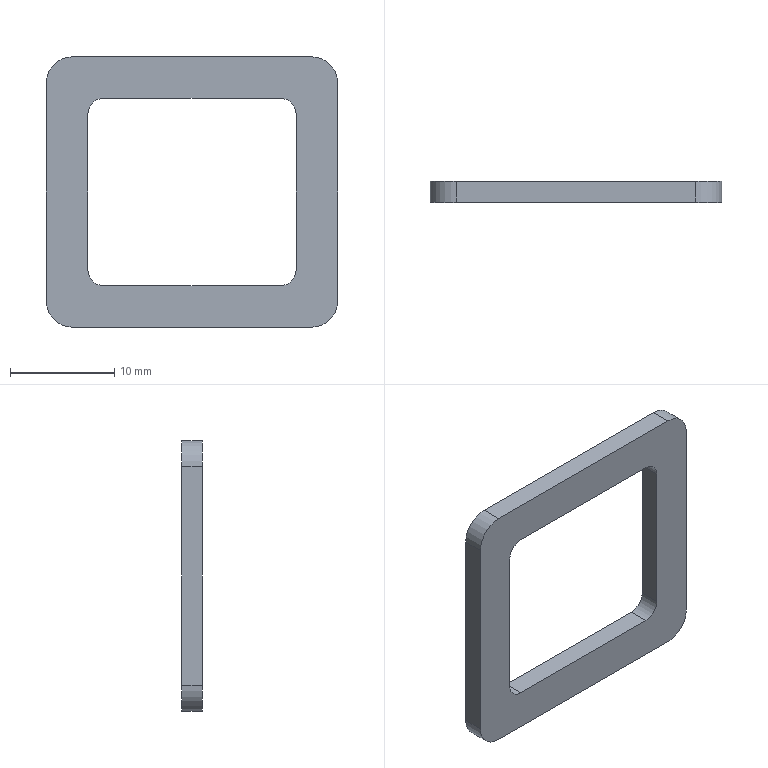Part | STEP file | 10000020460swp000-1 | 1 solid | 18 faces | box 28 x 2 x 26 mm | volume 729.133 mm3 | plane 10 | cylinder 8 | commonest cylinder face diameters 3 x4 5 x4
STEP:
#1=CARTESIAN_POINT('',(14.,2.,10.5));
#2=VERTEX_POINT('',#1);
#3=CARTESIAN_POINT('',(14.,2.,-10.5));
#4=VERTEX_POINT('',#3);
#5=CARTESIAN_POINT('',(14.,2.,-13.));
#6=DIRECTION('',(0.,0.,-1.));
#7=VECTOR('',#6,1000.);
#8=LINE('',#5,#7);
#9=EDGE_CURVE('',#2,#4,#8,.T.);
#10=ORIENTED_EDGE('',*,*,#9,.F.);
#11=CARTESIAN_POINT('',(14.,0.,10.5));
#12=VERTEX_POINT('',#11);
#13=CARTESIAN_POINT('',(14.,2.,10.5));
#14=DIRECTION('',(0.,-1.,0.));
#15=VECTOR('',#14,1000.);
#16=LINE('',#13,#15);
#17=EDGE_CURVE('',#2,#12,#16,.T.);
#18=ORIENTED_EDGE('',*,*,#17,.T.);
#19=CARTESIAN_POINT('',(14.,0.,-10.5));
#20=VERTEX_POINT('',#19);
#21=CARTESIAN_POINT('',(14.,0.,-13.));
#22=DIRECTION('',(0.,0.,-1.));
#23=VECTOR('',#22,1000.);
#24=LINE('',#21,#23);
#25=EDGE_CURVE('',#12,#20,#24,.T.);
#26=ORIENTED_EDGE('',*,*,#25,.T.);
#27=CARTESIAN_POINT('',(14.,2.,-10.5));
#28=DIRECTION('',(0.,1.,0.));
#29=VECTOR('',#28,1000.);
#30=LINE('',#27,#29);
#31=EDGE_CURVE('',#20,#4,#30,.T.);
#32=ORIENTED_EDGE('',*,*,#31,.T.);
#33=EDGE_LOOP('',(#10,#18,#26,#32));
#34=FACE_OUTER_BOUND('',#33,.T.);
#35=CARTESIAN_POINT('',(14.,2.,-13.));
#36=DIRECTION('',(-1.,0.,0.));
#37=DIRECTION('',(0.,0.,1.));
#38=AXIS2_PLACEMENT_3D('',#35,#36,#37);
#39=PLANE('',#38);
#40=ADVANCED_FACE('',(#34),#39,.F.);
#41=CARTESIAN_POINT('',(11.5,2.,-13.));
#42=VERTEX_POINT('',#41);
#43=CARTESIAN_POINT('',(-11.5,2.,-13.));
#44=VERTEX_POINT('',#43);
#45=CARTESIAN_POINT('',(-14.,2.,-13.));
#46=DIRECTION('',(-1.,0.,0.));
#47=VECTOR('',#46,1000.);
#48=LINE('',#45,#47);
#49=EDGE_CURVE('',#42,#44,#48,.T.);
#50=ORIENTED_EDGE('',*,*,#49,.F.);
#51=CARTESIAN_POINT('',(11.5,0.,-13.));
#52=VERTEX_POINT('',#51);
#53=CARTESIAN_POINT('',(11.5,2.,-13.));
#54=DIRECTION('',(0.,-1.,0.));
#55=VECTOR('',#54,1000.);
#56=LINE('',#53,#55);
#57=EDGE_CURVE('',#42,#52,#56,.T.);
#58=ORIENTED_EDGE('',*,*,#57,.T.);
#59=CARTESIAN_POINT('',(-11.5,0.,-13.));
#60=VERTEX_POINT('',#59);
#61=CARTESIAN_POINT('',(-14.,0.,-13.));
#62=DIRECTION('',(-1.,0.,0.));
#63=VECTOR('',#62,1000.);
#64=LINE('',#61,#63);
#65=EDGE_CURVE('',#52,#60,#64,.T.);
#66=ORIENTED_EDGE('',*,*,#65,.T.);
#67=CARTESIAN_POINT('',(-11.5,2.,-13.));
#68=DIRECTION('',(0.,1.,0.));
#69=VECTOR('',#68,1000.);
#70=LINE('',#67,#69);
#71=EDGE_CURVE('',#60,#44,#70,.T.);
#72=ORIENTED_EDGE('',*,*,#71,.T.);
#73=EDGE_LOOP('',(#50,#58,#66,#72));
#74=FACE_OUTER_BOUND('',#73,.T.);
#75=CARTESIAN_POINT('',(-14.,2.,-13.));
#76=DIRECTION('',(0.,0.,1.));
#77=DIRECTION('',(1.,0.,0.));
#78=AXIS2_PLACEMENT_3D('',#75,#76,#77);
#79=PLANE('',#78);
#80=ADVANCED_FACE('',(#74),#79,.F.);
#81=CARTESIAN_POINT('',(-14.,0.,-10.5));
#82=VERTEX_POINT('',#81);
#83=CARTESIAN_POINT('',(-14.,0.,10.5));
#84=VERTEX_POINT('',#83);
#85=CARTESIAN_POINT('',(-14.,0.,-13.));
#86=DIRECTION('',(0.,0.,1.));
#87=VECTOR('',#86,1000.);
#88=LINE('',#85,#87);
#89=EDGE_CURVE('',#82,#84,#88,.T.);
#90=ORIENTED_EDGE('',*,*,#89,.T.);
#91=CARTESIAN_POINT('',(-14.,2.,10.5));
#92=VERTEX_POINT('',#91);
#93=CARTESIAN_POINT('',(-14.,2.,10.5));
#94=DIRECTION('',(0.,1.,0.));
#95=VECTOR('',#94,1000.);
#96=LINE('',#93,#95);
#97=EDGE_CURVE('',#84,#92,#96,.T.);
#98=ORIENTED_EDGE('',*,*,#97,.T.);
#99=CARTESIAN_POINT('',(-14.,2.,-10.5));
#100=VERTEX_POINT('',#99);
#101=CARTESIAN_POINT('',(-14.,2.,-13.));
#102=DIRECTION('',(0.,0.,1.));
#103=VECTOR('',#102,1000.);
#104=LINE('',#101,#103);
#105=EDGE_CURVE('',#100,#92,#104,.T.);
#106=ORIENTED_EDGE('',*,*,#105,.F.);
#107=CARTESIAN_POINT('',(-14.,2.,-10.5));
#108=DIRECTION('',(0.,-1.,0.));
#109=VECTOR('',#108,1000.);
#110=LINE('',#107,#109);
#111=EDGE_CURVE('',#100,#82,#110,.T.);
#112=ORIENTED_EDGE('',*,*,#111,.T.);
#113=EDGE_LOOP('',(#90,#98,#106,#112));
#114=FACE_OUTER_BOUND('',#113,.T.);
#115=CARTESIAN_POINT('',(-14.,2.,-13.));
#116=DIRECTION('',(1.,0.,0.));
#117=DIRECTION('',(0.,0.,-1.));
#118=AXIS2_PLACEMENT_3D('',#115,#116,#117);
#119=PLANE('',#118);
#120=ADVANCED_FACE('',(#114),#119,.F.);
#121=CARTESIAN_POINT('',(-11.5,0.,13.));
#122=VERTEX_POINT('',#121);
#123=CARTESIAN_POINT('',(11.5,0.,13.));
#124=VERTEX_POINT('',#123);
#125=CARTESIAN_POINT('',(-14.,0.,13.));
#126=DIRECTION('',(1.,0.,0.));
#127=VECTOR('',#126,1000.);
#128=LINE('',#125,#127);
#129=EDGE_CURVE('',#122,#124,#128,.T.);
#130=ORIENTED_EDGE('',*,*,#129,.T.);
#131=CARTESIAN_POINT('',(11.5,2.,13.));
#132=VERTEX_POINT('',#131);
#133=CARTESIAN_POINT('',(11.5,2.,13.));
#134=DIRECTION('',(0.,1.,0.));
#135=VECTOR('',#134,1000.);
#136=LINE('',#133,#135);
#137=EDGE_CURVE('',#124,#132,#136,.T.);
#138=ORIENTED_EDGE('',*,*,#137,.T.);
#139=CARTESIAN_POINT('',(-11.5,2.,13.));
#140=VERTEX_POINT('',#139);
#141=CARTESIAN_POINT('',(-14.,2.,13.));
#142=DIRECTION('',(1.,0.,0.));
#143=VECTOR('',#142,1000.);
#144=LINE('',#141,#143);
#145=EDGE_CURVE('',#140,#132,#144,.T.);
#146=ORIENTED_EDGE('',*,*,#145,.F.);
#147=CARTESIAN_POINT('',(-11.5,2.,13.));
#148=DIRECTION('',(0.,-1.,0.));
#149=VECTOR('',#148,1000.);
#150=LINE('',#147,#149);
#151=EDGE_CURVE('',#140,#122,#150,.T.);
#152=ORIENTED_EDGE('',*,*,#151,.T.);
#153=EDGE_LOOP('',(#130,#138,#146,#152));
#154=FACE_OUTER_BOUND('',#153,.T.);
#155=CARTESIAN_POINT('',(-14.,2.,13.));
#156=DIRECTION('',(0.,0.,-1.));
#157=DIRECTION('',(-1.,0.,0.));
#158=AXIS2_PLACEMENT_3D('',#155,#156,#157);
#159=PLANE('',#158);
#160=ADVANCED_FACE('',(#154),#159,.F.);
#161=CARTESIAN_POINT('',(-8.5,2.,9.));
#162=VERTEX_POINT('',#161);
#163=CARTESIAN_POINT('',(8.5,2.,9.));
#164=VERTEX_POINT('',#163);
#165=CARTESIAN_POINT('',(-10.,2.,9.));
#166=DIRECTION('',(1.,0.,0.));
#167=VECTOR('',#166,1000.);
#168=LINE('',#165,#167);
#169=EDGE_CURVE('',#162,#164,#168,.T.);
#170=ORIENTED_EDGE('',*,*,#169,.F.);
#171=CARTESIAN_POINT('',(-10.,2.,7.5));
#172=VERTEX_POINT('',#171);
#173=CARTESIAN_POINT('',(-8.5,2.,7.5));
#174=DIRECTION('',(0.,-1.,0.));
#175=DIRECTION('',(0.,0.,1.));
#176=AXIS2_PLACEMENT_3D('',#173,#174,#175);
#177=CIRCLE('',#176,1.5);
#178=EDGE_CURVE('',#162,#172,#177,.T.);
#179=ORIENTED_EDGE('',*,*,#178,.T.);
#180=CARTESIAN_POINT('',(-10.,2.,-7.5));
#181=VERTEX_POINT('',#180);
#182=CARTESIAN_POINT('',(-10.,2.,-9.));
#183=DIRECTION('',(0.,0.,1.));
#184=VECTOR('',#183,1000.);
#185=LINE('',#182,#184);
#186=EDGE_CURVE('',#181,#172,#185,.T.);
#187=ORIENTED_EDGE('',*,*,#186,.F.);
#188=CARTESIAN_POINT('',(-8.5,2.,-9.));
#189=VERTEX_POINT('',#188);
#190=CARTESIAN_POINT('',(-8.5,2.,-7.5));
#191=DIRECTION('',(0.,-1.,0.));
#192=DIRECTION('',(0.,0.,1.));
#193=AXIS2_PLACEMENT_3D('',#190,#191,#192);
#194=CIRCLE('',#193,1.5);
#195=EDGE_CURVE('',#181,#189,#194,.T.);
#196=ORIENTED_EDGE('',*,*,#195,.T.);
#197=CARTESIAN_POINT('',(8.5,2.,-9.));
#198=VERTEX_POINT('',#197);
#199=CARTESIAN_POINT('',(10.,2.,-9.));
#200=DIRECTION('',(-1.,0.,0.));
#201=VECTOR('',#200,1000.);
#202=LINE('',#199,#201);
#203=EDGE_CURVE('',#198,#189,#202,.T.);
#204=ORIENTED_EDGE('',*,*,#203,.F.);
#205=CARTESIAN_POINT('',(10.,2.,-7.5));
#206=VERTEX_POINT('',#205);
#207=CARTESIAN_POINT('',(8.5,2.,-7.5));
#208=DIRECTION('',(0.,-1.,0.));
#209=DIRECTION('',(0.,0.,1.));
#210=AXIS2_PLACEMENT_3D('',#207,#208,#209);
#211=CIRCLE('',#210,1.5);
#212=EDGE_CURVE('',#198,#206,#211,.T.);
#213=ORIENTED_EDGE('',*,*,#212,.T.);
#214=CARTESIAN_POINT('',(10.,2.,7.5));
#215=VERTEX_POINT('',#214);
#216=CARTESIAN_POINT('',(10.,2.,9.));
#217=DIRECTION('',(0.,0.,-1.));
#218=VECTOR('',#217,1000.);
#219=LINE('',#216,#218);
#220=EDGE_CURVE('',#215,#206,#219,.T.);
#221=ORIENTED_EDGE('',*,*,#220,.F.);
#222=CARTESIAN_POINT('',(8.5,2.,7.5));
#223=DIRECTION('',(0.,-1.,0.));
#224=DIRECTION('',(0.,0.,1.));
#225=AXIS2_PLACEMENT_3D('',#222,#223,#224);
#226=CIRCLE('',#225,1.5);
#227=EDGE_CURVE('',#215,#164,#226,.T.);
#228=ORIENTED_EDGE('',*,*,#227,.T.);
#229=EDGE_LOOP('',(#170,#179,#187,#196,#204,#213,#221,#228));
#230=FACE_BOUND('',#229,.T.);
#231=ORIENTED_EDGE('',*,*,#145,.T.);
#232=CARTESIAN_POINT('',(11.5,2.,10.5));
#233=DIRECTION('',(0.,1.,0.));
#234=DIRECTION('',(0.,0.,1.));
#235=AXIS2_PLACEMENT_3D('',#232,#233,#234);
#236=CIRCLE('',#235,2.5);
#237=EDGE_CURVE('',#132,#2,#236,.T.);
#238=ORIENTED_EDGE('',*,*,#237,.T.);
#239=ORIENTED_EDGE('',*,*,#9,.T.);
#240=CARTESIAN_POINT('',(11.5,2.,-10.5));
#241=DIRECTION('',(0.,1.,0.));
#242=DIRECTION('',(0.,0.,1.));
#243=AXIS2_PLACEMENT_3D('',#240,#241,#242);
#244=CIRCLE('',#243,2.5);
#245=EDGE_CURVE('',#4,#42,#244,.T.);
#246=ORIENTED_EDGE('',*,*,#245,.T.);
#247=ORIENTED_EDGE('',*,*,#49,.T.);
#248=CARTESIAN_POINT('',(-11.5,2.,-10.5));
#249=DIRECTION('',(0.,1.,0.));
#250=DIRECTION('',(0.,0.,1.));
#251=AXIS2_PLACEMENT_3D('',#248,#249,#250);
#252=CIRCLE('',#251,2.5);
#253=EDGE_CURVE('',#44,#100,#252,.T.);
#254=ORIENTED_EDGE('',*,*,#253,.T.);
#255=ORIENTED_EDGE('',*,*,#105,.T.);
#256=CARTESIAN_POINT('',(-11.5,2.,10.5));
#257=DIRECTION('',(0.,1.,0.));
#258=DIRECTION('',(0.,0.,1.));
#259=AXIS2_PLACEMENT_3D('',#256,#257,#258);
#260=CIRCLE('',#259,2.5);
#261=EDGE_CURVE('',#92,#140,#260,.T.);
#262=ORIENTED_EDGE('',*,*,#261,.T.);
#263=EDGE_LOOP('',(#231,#238,#239,#246,#247,#254,#255,#262));
#264=FACE_OUTER_BOUND('',#263,.T.);
#265=CARTESIAN_POINT('',(0.,2.,0.));
#266=DIRECTION('',(0.,1.,0.));
#267=DIRECTION('',(0.,0.,1.));
#268=AXIS2_PLACEMENT_3D('',#265,#266,#267);
#269=PLANE('',#268);
#270=ADVANCED_FACE('',(#230,#264),#269,.T.);
#271=CARTESIAN_POINT('',(8.5,0.,-9.));
#272=VERTEX_POINT('',#271);
#273=CARTESIAN_POINT('',(-8.5,0.,-9.));
#274=VERTEX_POINT('',#273);
#275=CARTESIAN_POINT('',(10.,0.,-9.));
#276=DIRECTION('',(-1.,0.,0.));
#277=VECTOR('',#276,1000.);
#278=LINE('',#275,#277);
#279=EDGE_CURVE('',#272,#274,#278,.T.);
#280=ORIENTED_EDGE('',*,*,#279,.T.);
#281=CARTESIAN_POINT('',(-10.,0.,-7.5));
#282=VERTEX_POINT('',#281);
#283=CARTESIAN_POINT('',(-8.5,0.,-7.5));
#284=DIRECTION('',(0.,1.,0.));
#285=DIRECTION('',(0.,0.,1.));
#286=AXIS2_PLACEMENT_3D('',#283,#284,#285);
#287=CIRCLE('',#286,1.5);
#288=EDGE_CURVE('',#274,#282,#287,.T.);
#289=ORIENTED_EDGE('',*,*,#288,.T.);
#290=CARTESIAN_POINT('',(-10.,0.,7.5));
#291=VERTEX_POINT('',#290);
#292=CARTESIAN_POINT('',(-10.,0.,-9.));
#293=DIRECTION('',(0.,0.,1.));
#294=VECTOR('',#293,1000.);
#295=LINE('',#292,#294);
#296=EDGE_CURVE('',#282,#291,#295,.T.);
#297=ORIENTED_EDGE('',*,*,#296,.T.);
#298=CARTESIAN_POINT('',(-8.5,0.,9.));
#299=VERTEX_POINT('',#298);
#300=CARTESIAN_POINT('',(-8.5,0.,7.5));
#301=DIRECTION('',(0.,1.,0.));
#302=DIRECTION('',(0.,0.,1.));
#303=AXIS2_PLACEMENT_3D('',#300,#301,#302);
#304=CIRCLE('',#303,1.5);
#305=EDGE_CURVE('',#291,#299,#304,.T.);
#306=ORIENTED_EDGE('',*,*,#305,.T.);
#307=CARTESIAN_POINT('',(8.5,0.,9.));
#308=VERTEX_POINT('',#307);
#309=CARTESIAN_POINT('',(-10.,0.,9.));
#310=DIRECTION('',(1.,0.,0.));
#311=VECTOR('',#310,1000.);
#312=LINE('',#309,#311);
#313=EDGE_CURVE('',#299,#308,#312,.T.);
#314=ORIENTED_EDGE('',*,*,#313,.T.);
#315=CARTESIAN_POINT('',(10.,0.,7.5));
#316=VERTEX_POINT('',#315);
#317=CARTESIAN_POINT('',(8.5,0.,7.5));
#318=DIRECTION('',(0.,1.,0.));
#319=DIRECTION('',(0.,0.,1.));
#320=AXIS2_PLACEMENT_3D('',#317,#318,#319);
#321=CIRCLE('',#320,1.5);
#322=EDGE_CURVE('',#308,#316,#321,.T.);
#323=ORIENTED_EDGE('',*,*,#322,.T.);
#324=CARTESIAN_POINT('',(10.,0.,-7.5));
#325=VERTEX_POINT('',#324);
#326=CARTESIAN_POINT('',(10.,0.,9.));
#327=DIRECTION('',(0.,0.,-1.));
#328=VECTOR('',#327,1000.);
#329=LINE('',#326,#328);
#330=EDGE_CURVE('',#316,#325,#329,.T.);
#331=ORIENTED_EDGE('',*,*,#330,.T.);
#332=CARTESIAN_POINT('',(8.5,0.,-7.5));
#333=DIRECTION('',(0.,1.,0.));
#334=DIRECTION('',(0.,0.,1.));
#335=AXIS2_PLACEMENT_3D('',#332,#333,#334);
#336=CIRCLE('',#335,1.5);
#337=EDGE_CURVE('',#325,#272,#336,.T.);
#338=ORIENTED_EDGE('',*,*,#337,.T.);
#339=EDGE_LOOP('',(#280,#289,#297,#306,#314,#323,#331,#338));
#340=FACE_BOUND('',#339,.T.);
#341=ORIENTED_EDGE('',*,*,#25,.F.);
#342=CARTESIAN_POINT('',(11.5,0.,10.5));
#343=DIRECTION('',(0.,-1.,0.));
#344=DIRECTION('',(0.,0.,1.));
#345=AXIS2_PLACEMENT_3D('',#342,#343,#344);
#346=CIRCLE('',#345,2.5);
#347=EDGE_CURVE('',#12,#124,#346,.T.);
#348=ORIENTED_EDGE('',*,*,#347,.T.);
#349=ORIENTED_EDGE('',*,*,#129,.F.);
#350=CARTESIAN_POINT('',(-11.5,0.,10.5));
#351=DIRECTION('',(0.,-1.,0.));
#352=DIRECTION('',(0.,0.,1.));
#353=AXIS2_PLACEMENT_3D('',#350,#351,#352);
#354=CIRCLE('',#353,2.5);
#355=EDGE_CURVE('',#122,#84,#354,.T.);
#356=ORIENTED_EDGE('',*,*,#355,.T.);
#357=ORIENTED_EDGE('',*,*,#89,.F.);
#358=CARTESIAN_POINT('',(-11.5,0.,-10.5));
#359=DIRECTION('',(0.,-1.,0.));
#360=DIRECTION('',(0.,0.,1.));
#361=AXIS2_PLACEMENT_3D('',#358,#359,#360);
#362=CIRCLE('',#361,2.5);
#363=EDGE_CURVE('',#82,#60,#362,.T.);
#364=ORIENTED_EDGE('',*,*,#363,.T.);
#365=ORIENTED_EDGE('',*,*,#65,.F.);
#366=CARTESIAN_POINT('',(11.5,0.,-10.5));
#367=DIRECTION('',(0.,-1.,0.));
#368=DIRECTION('',(0.,0.,1.));
#369=AXIS2_PLACEMENT_3D('',#366,#367,#368);
#370=CIRCLE('',#369,2.5);
#371=EDGE_CURVE('',#52,#20,#370,.T.);
#372=ORIENTED_EDGE('',*,*,#371,.T.);
#373=EDGE_LOOP('',(#341,#348,#349,#356,#357,#364,#365,#372));
#374=FACE_OUTER_BOUND('',#373,.T.);
#375=CARTESIAN_POINT('',(0.,0.,0.));
#376=DIRECTION('',(0.,1.,0.));
#377=DIRECTION('',(0.,0.,1.));
#378=AXIS2_PLACEMENT_3D('',#375,#376,#377);
#379=PLANE('',#378);
#380=ADVANCED_FACE('',(#340,#374),#379,.F.);
#381=ORIENTED_EDGE('',*,*,#313,.F.);
#382=CARTESIAN_POINT('',(-8.5,2.,9.));
#383=DIRECTION('',(0.,1.,0.));
#384=VECTOR('',#383,1000.);
#385=LINE('',#382,#384);
#386=EDGE_CURVE('',#299,#162,#385,.T.);
#387=ORIENTED_EDGE('',*,*,#386,.T.);
#388=ORIENTED_EDGE('',*,*,#169,.T.);
#389=CARTESIAN_POINT('',(8.5,0.,9.));
#390=DIRECTION('',(0.,-1.,0.));
#391=VECTOR('',#390,1000.);
#392=LINE('',#389,#391);
#393=EDGE_CURVE('',#164,#308,#392,.T.);
#394=ORIENTED_EDGE('',*,*,#393,.T.);
#395=EDGE_LOOP('',(#381,#387,#388,#394));
#396=FACE_OUTER_BOUND('',#395,.T.);
#397=CARTESIAN_POINT('',(-10.,0.,9.));
#398=DIRECTION('',(0.,0.,1.));
#399=DIRECTION('',(1.,0.,0.));
#400=AXIS2_PLACEMENT_3D('',#397,#398,#399);
#401=PLANE('',#400);
#402=ADVANCED_FACE('',(#396),#401,.F.);
#403=ORIENTED_EDGE('',*,*,#186,.T.);
#404=CARTESIAN_POINT('',(-10.,0.,7.5));
#405=DIRECTION('',(0.,-1.,0.));
#406=VECTOR('',#405,1000.);
#407=LINE('',#404,#406);
#408=EDGE_CURVE('',#172,#291,#407,.T.);
#409=ORIENTED_EDGE('',*,*,#408,.T.);
#410=ORIENTED_EDGE('',*,*,#296,.F.);
#411=CARTESIAN_POINT('',(-10.,2.,-7.5));
#412=DIRECTION('',(0.,1.,0.));
#413=VECTOR('',#412,1000.);
#414=LINE('',#411,#413);
#415=EDGE_CURVE('',#282,#181,#414,.T.);
#416=ORIENTED_EDGE('',*,*,#415,.T.);
#417=EDGE_LOOP('',(#403,#409,#410,#416));
#418=FACE_OUTER_BOUND('',#417,.T.);
#419=CARTESIAN_POINT('',(-10.,0.,-9.));
#420=DIRECTION('',(-1.,0.,0.));
#421=DIRECTION('',(0.,0.,1.));
#422=AXIS2_PLACEMENT_3D('',#419,#420,#421);
#423=PLANE('',#422);
#424=ADVANCED_FACE('',(#418),#423,.F.);
#425=ORIENTED_EDGE('',*,*,#279,.F.);
#426=CARTESIAN_POINT('',(8.5,2.,-9.));
#427=DIRECTION('',(0.,1.,0.));
#428=VECTOR('',#427,1000.);
#429=LINE('',#426,#428);
#430=EDGE_CURVE('',#272,#198,#429,.T.);
#431=ORIENTED_EDGE('',*,*,#430,.T.);
#432=ORIENTED_EDGE('',*,*,#203,.T.);
#433=CARTESIAN_POINT('',(-8.5,0.,-9.));
#434=DIRECTION('',(0.,-1.,0.));
#435=VECTOR('',#434,1000.);
#436=LINE('',#433,#435);
#437=EDGE_CURVE('',#189,#274,#436,.T.);
#438=ORIENTED_EDGE('',*,*,#437,.T.);
#439=EDGE_LOOP('',(#425,#431,#432,#438));
#440=FACE_OUTER_BOUND('',#439,.T.);
#441=CARTESIAN_POINT('',(10.,0.,-9.));
#442=DIRECTION('',(0.,0.,-1.));
#443=DIRECTION('',(-1.,0.,0.));
#444=AXIS2_PLACEMENT_3D('',#441,#442,#443);
#445=PLANE('',#444);
#446=ADVANCED_FACE('',(#440),#445,.F.);
#447=ORIENTED_EDGE('',*,*,#330,.F.);
#448=CARTESIAN_POINT('',(10.,2.,7.5));
#449=DIRECTION('',(0.,1.,0.));
#450=VECTOR('',#449,1000.);
#451=LINE('',#448,#450);
#452=EDGE_CURVE('',#316,#215,#451,.T.);
#453=ORIENTED_EDGE('',*,*,#452,.T.);
#454=ORIENTED_EDGE('',*,*,#220,.T.);
#455=CARTESIAN_POINT('',(10.,0.,-7.5));
#456=DIRECTION('',(0.,-1.,0.));
#457=VECTOR('',#456,1000.);
#458=LINE('',#455,#457);
#459=EDGE_CURVE('',#206,#325,#458,.T.);
#460=ORIENTED_EDGE('',*,*,#459,.T.);
#461=EDGE_LOOP('',(#447,#453,#454,#460));
#462=FACE_OUTER_BOUND('',#461,.T.);
#463=CARTESIAN_POINT('',(10.,0.,9.));
#464=DIRECTION('',(1.,0.,0.));
#465=DIRECTION('',(0.,0.,-1.));
#466=AXIS2_PLACEMENT_3D('',#463,#464,#465);
#467=PLANE('',#466);
#468=ADVANCED_FACE('',(#462),#467,.F.);
#469=ORIENTED_EDGE('',*,*,#237,.F.);
#470=ORIENTED_EDGE('',*,*,#137,.F.);
#471=ORIENTED_EDGE('',*,*,#347,.F.);
#472=ORIENTED_EDGE('',*,*,#17,.F.);
#473=EDGE_LOOP('',(#469,#470,#471,#472));
#474=FACE_OUTER_BOUND('',#473,.T.);
#475=CARTESIAN_POINT('',(11.5,2.,10.5));
#476=DIRECTION('',(0.,-1.,0.));
#477=DIRECTION('',(0.,0.,-1.));
#478=AXIS2_PLACEMENT_3D('',#475,#476,#477);
#479=CYLINDRICAL_SURFACE('',#478,2.5);
#480=ADVANCED_FACE('',(#474),#479,.T.);
#481=ORIENTED_EDGE('',*,*,#261,.F.);
#482=ORIENTED_EDGE('',*,*,#97,.F.);
#483=ORIENTED_EDGE('',*,*,#355,.F.);
#484=ORIENTED_EDGE('',*,*,#151,.F.);
#485=EDGE_LOOP('',(#481,#482,#483,#484));
#486=FACE_OUTER_BOUND('',#485,.T.);
#487=CARTESIAN_POINT('',(-11.5,2.,10.5));
#488=DIRECTION('',(0.,-1.,0.));
#489=DIRECTION('',(0.,0.,-1.));
#490=AXIS2_PLACEMENT_3D('',#487,#488,#489);
#491=CYLINDRICAL_SURFACE('',#490,2.5);
#492=ADVANCED_FACE('',(#486),#491,.T.);
#493=ORIENTED_EDGE('',*,*,#245,.F.);
#494=ORIENTED_EDGE('',*,*,#31,.F.);
#495=ORIENTED_EDGE('',*,*,#371,.F.);
#496=ORIENTED_EDGE('',*,*,#57,.F.);
#497=EDGE_LOOP('',(#493,#494,#495,#496));
#498=FACE_OUTER_BOUND('',#497,.T.);
#499=CARTESIAN_POINT('',(11.5,2.,-10.5));
#500=DIRECTION('',(0.,-1.,0.));
#501=DIRECTION('',(0.,0.,-1.));
#502=AXIS2_PLACEMENT_3D('',#499,#500,#501);
#503=CYLINDRICAL_SURFACE('',#502,2.5);
#504=ADVANCED_FACE('',(#498),#503,.T.);
#505=ORIENTED_EDGE('',*,*,#253,.F.);
#506=ORIENTED_EDGE('',*,*,#71,.F.);
#507=ORIENTED_EDGE('',*,*,#363,.F.);
#508=ORIENTED_EDGE('',*,*,#111,.F.);
#509=EDGE_LOOP('',(#505,#506,#507,#508));
#510=FACE_OUTER_BOUND('',#509,.T.);
#511=CARTESIAN_POINT('',(-11.5,2.,-10.5));
#512=DIRECTION('',(0.,-1.,0.));
#513=DIRECTION('',(0.,0.,-1.));
#514=AXIS2_PLACEMENT_3D('',#511,#512,#513);
#515=CYLINDRICAL_SURFACE('',#514,2.5);
#516=ADVANCED_FACE('',(#510),#515,.T.);
#517=ORIENTED_EDGE('',*,*,#305,.F.);
#518=ORIENTED_EDGE('',*,*,#408,.F.);
#519=ORIENTED_EDGE('',*,*,#178,.F.);
#520=ORIENTED_EDGE('',*,*,#386,.F.);
#521=EDGE_LOOP('',(#517,#518,#519,#520));
#522=FACE_OUTER_BOUND('',#521,.T.);
#523=CARTESIAN_POINT('',(-8.5,0.,7.5));
#524=DIRECTION('',(0.,-1.,0.));
#525=DIRECTION('',(0.,0.,-1.));
#526=AXIS2_PLACEMENT_3D('',#523,#524,#525);
#527=CYLINDRICAL_SURFACE('',#526,1.5);
#528=ADVANCED_FACE('',(#522),#527,.F.);
#529=ORIENTED_EDGE('',*,*,#322,.F.);
#530=ORIENTED_EDGE('',*,*,#393,.F.);
#531=ORIENTED_EDGE('',*,*,#227,.F.);
#532=ORIENTED_EDGE('',*,*,#452,.F.);
#533=EDGE_LOOP('',(#529,#530,#531,#532));
#534=FACE_OUTER_BOUND('',#533,.T.);
#535=CARTESIAN_POINT('',(8.5,0.,7.5));
#536=DIRECTION('',(0.,-1.,0.));
#537=DIRECTION('',(0.,0.,-1.));
#538=AXIS2_PLACEMENT_3D('',#535,#536,#537);
#539=CYLINDRICAL_SURFACE('',#538,1.5);
#540=ADVANCED_FACE('',(#534),#539,.F.);
#541=ORIENTED_EDGE('',*,*,#337,.F.);
#542=ORIENTED_EDGE('',*,*,#459,.F.);
#543=ORIENTED_EDGE('',*,*,#212,.F.);
#544=ORIENTED_EDGE('',*,*,#430,.F.);
#545=EDGE_LOOP('',(#541,#542,#543,#544));
#546=FACE_OUTER_BOUND('',#545,.T.);
#547=CARTESIAN_POINT('',(8.5,0.,-7.5));
#548=DIRECTION('',(0.,-1.,0.));
#549=DIRECTION('',(0.,0.,-1.));
#550=AXIS2_PLACEMENT_3D('',#547,#548,#549);
#551=CYLINDRICAL_SURFACE('',#550,1.5);
#552=ADVANCED_FACE('',(#546),#551,.F.);
#553=ORIENTED_EDGE('',*,*,#288,.F.);
#554=ORIENTED_EDGE('',*,*,#437,.F.);
#555=ORIENTED_EDGE('',*,*,#195,.F.);
#556=ORIENTED_EDGE('',*,*,#415,.F.);
#557=EDGE_LOOP('',(#553,#554,#555,#556));
#558=FACE_OUTER_BOUND('',#557,.T.);
#559=CARTESIAN_POINT('',(-8.5,0.,-7.5));
#560=DIRECTION('',(0.,-1.,0.));
#561=DIRECTION('',(0.,0.,-1.));
#562=AXIS2_PLACEMENT_3D('',#559,#560,#561);
#563=CYLINDRICAL_SURFACE('',#562,1.5);
#564=ADVANCED_FACE('',(#558),#563,.F.);
#565=CLOSED_SHELL('',(#40,#80,#120,#160,#270,#380,#402,#424,#446,#468,#480,#492,#504,#516,#528,#540,#552,#564));
#566=MANIFOLD_SOLID_BREP('',#565);
#567=CARTESIAN_POINT('',(0.,0.,0.));
#568=DIRECTION('',(0.,0.,1.));
#569=DIRECTION('',(1.,0.,0.));
#570=AXIS2_PLACEMENT_3D('',#567,#568,#569);
#571=(LENGTH_UNIT()NAMED_UNIT(*)SI_UNIT(.MILLI.,.METRE.));
#572=UNCERTAINTY_MEASURE_WITH_UNIT(LENGTH_MEASURE(0.00001),#571,'','');
#573=(NAMED_UNIT(*)PLANE_ANGLE_UNIT()SI_UNIT($,.RADIAN.));
#574=(NAMED_UNIT(*)SI_UNIT($,.STERADIAN.)SOLID_ANGLE_UNIT());
#575=(GEOMETRIC_REPRESENTATION_CONTEXT(3)GLOBAL_UNCERTAINTY_ASSIGNED_CONTEXT((#572))GLOBAL_UNIT_ASSIGNED_CONTEXT((#571,#573,#574))REPRESENTATION_CONTEXT('',''));
#576=ADVANCED_BREP_SHAPE_REPRESENTATION('',(#566,#570),#575);